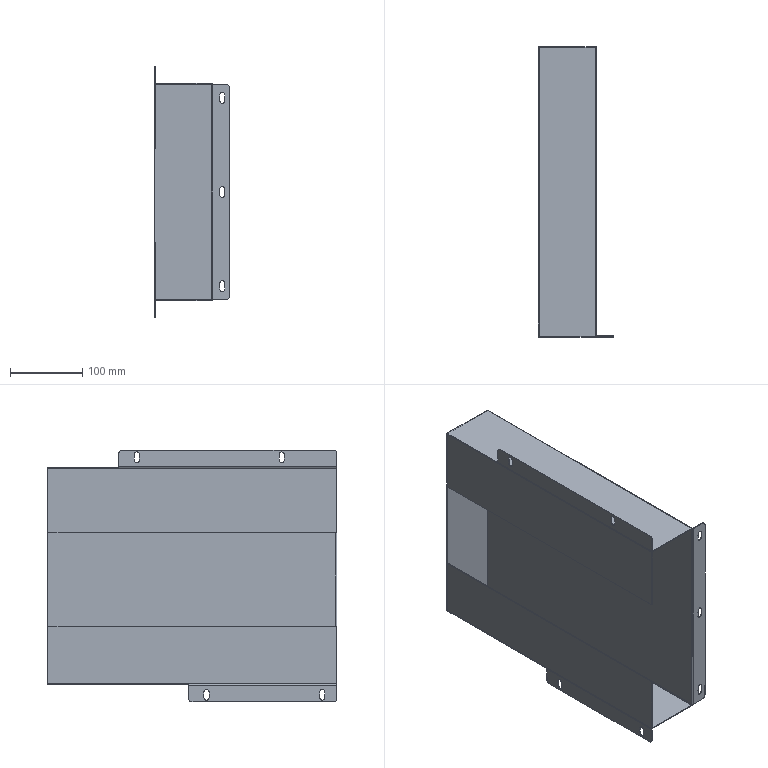Part | SolidWorks | features BaseBody 4 | 4 solids | 114 faces | box 103.8 x 400 x 347.6 mm | volume 349183 mm3 | plane 78 | cylinder 36 | commonest cylinder face diameters 7 x18 1 x7 10 x6 3.4 x5